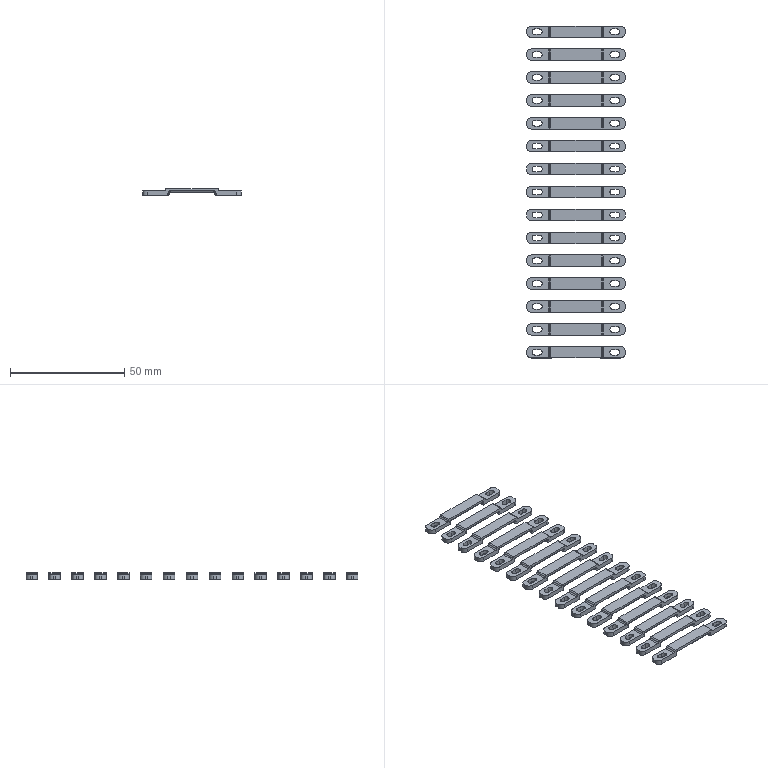NC program | NX | posted with a generic post | part box 43 x 145 x 3 mm
Whole program:
N10 G17 G21 G94 G90
(FLOOR_WALL_COPY , TOOL : D10JING)
N12 T15 M6
N14 G54
N16 G17 G0 G90 X29.5 Y0. S6500 M3
N18 G43 Z30. H15
N20 Z3.
N22 G94 G1 Z0. F1500.
N24 X26.5
N26 X-26.5
N28 X-29.5
N30 Z3.
N32 G0 Z30.
N34 M5
(FLOOR_WALL_1_COPY_1 , TOOL : D4)
N36 T11 M6
N38 G54
N40 G17 G0 G90 X-24.409 Y-1.452 S9500 M3
N42 G43 Z30. H11
N44 Z1.075
N46 G94 G1 Z0.075 F1000.
N48 X-23.643 Y-0.81
N50 G3 X-23.5 Y-0.503 R0.4
N52 G1 Y0.503 F2500.
N54 G2 X-21.075 Y4.177 R4.
N56 G1 Y-4.177
N58 G3 X-19.5 Y-4.5 R4.
N60 G1 X-18.65
N62 Y4.5
N64 X-16.225
N66 Y-4.5
N68 X-13.8
N70 Y4.5
N72 G3 X-13.943 Y4.806 R0.4
N74 G1 X-14.769 Y5.5
N76 Z1.075
N78 G0 X-24.409 Y-1.452 Z0.75
N80 G1 Z-0.25 F1000.
N82 X-23.643 Y-0.81
N84 G3 X-23.5 Y-0.503 R0.4
N86 G1 Y0.503 F2500.
N88 G2 X-21.075 Y4.177 R4.
N90 G1 Y-4.177
N92 G3 X-19.5 Y-4.5 R4.
N94 G1 X-18.65
N96 Y4.5
N98 X-16.225
N100 Y-4.5
N102 X-13.8
N104 Y4.5
N106 G3 X-13.943 Y4.806 R0.4
N108 G1 X-14.769 Y5.5
N110 Z0.75
N112 G0 X-24.409 Y-1.452 Z0.425
N114 G1 Z-0.575 F1000.
N116 X-23.643 Y-0.81
N118 G3 X-23.5 Y-0.503 R0.4
N120 G1 Y0.503 F2500.
N122 G2 X-21.075 Y4.177 R4.
N124 G1 Y-4.177
N126 G3 X-19.5 Y-4.5 R4.
N128 G1 X-18.65
N130 Y4.5
N132 X-16.225
N134 Y-4.5
N136 X-13.8
N138 Y4.5
N140 G3 X-13.943 Y4.806 R0.4
N142 G1 X-14.769 Y5.5
N144 Z0.425
N146 G0 Z30.
N148 X-24.402 Y-1.484
N150 Z0.1
N152 G1 Z-0.9 F1000.
N154 X-23.641 Y-0.836
N156 G3 X-23.5 Y-0.529 R0.4
N158 G1 Y-0.521 F2500.
N160 Y-0.5
N162 Y0.5
N164 G2 X-21.228 Y4.108 R4.
N166 G1 X-21.176 Y-4.132
N168 G3 X-19.5 Y-4.5 R4.
N170 G1 X-18.872
N172 X-18.929 Y4.5
N174 X-16.628
N176 X-16.571 Y-4.5
N178 X-14.269
N180 X-14.279 Y-2.97
N182 G3 X-14.424 Y-2.664 R0.4
N184 G1 X-14.8 Y-5.5
N186 Z0.1
N188 G0 Z30.
N190 X-14.322 Y-0.35
N192 Z0.425
N194 G1 X-14.3 Y2.922 Z-0.452 F1000.
N196 X-13.976 Y3.233 Z-0.572
N198 X-13.8 Y3.231 Z-0.619
N200 X-13.976 Y3.233 Z-0.666
N202 X-14.3 Y2.922 Z-0.787
N204 X-14.314 Y2.5 Z-0.9
N206 X-14.326 Y4.5 F2500.
N208 G3 X-14.471 Y4.806 R0.4
N210 G1 X-15.309 Y5.5
N212 Z0.1
N214 G0 Z30.
N216 X24.409 Y1.452
N218 Z1.075
N220 G1 Z0.075 F1000.
N222 X23.643 Y0.81
N224 G3 X23.5 Y0.503 R0.4
N226 G1 Y-0.503 F2500.
N228 G2 X21.075 Y-4.177 R4.
N230 G1 Y4.177
N232 G3 X19.5 Y4.5 R4.
N234 G1 X18.65
N236 Y-4.5
N238 X16.225
N240 Y4.5
N242 X13.8
N244 Y-4.5
N246 G3 X13.943 Y-4.806 R0.4
N248 G1 X14.769 Y-5.5
N250 Z1.075
N252 G0 X24.409 Y1.452 Z0.75
N254 G1 Z-0.25 F1000.
N256 X23.643 Y0.81
N258 G3 X23.5 Y0.503 R0.4
N260 G1 Y-0.503 F2500.
N262 G2 X21.075 Y-4.177 R4.
N264 G1 Y4.177
N266 G3 X19.5 Y4.5 R4.
N268 G1 X18.65
N270 Y-4.5
N272 X16.225
N274 Y4.5
N276 X13.8
N278 Y-4.5
N280 G3 X13.943 Y-4.806 R0.4
N282 G1 X14.769 Y-5.5
N284 Z0.75
N286 G0 X24.409 Y1.452 Z0.425
N288 G1 Z-0.575 F1000.
N290 X23.643 Y0.81
N292 G3 X23.5 Y0.503 R0.4
N294 G1 Y-0.503 F2500.
N296 G2 X21.075 Y-4.177 R4.
N298 G1 Y4.177
N300 G3 X19.5 Y4.5 R4.
N302 G1 X18.65
N304 Y-4.5
N306 X16.225
N308 Y4.5
N310 X13.8
N312 Y-4.5
N314 G3 X13.943 Y-4.806 R0.4
N316 G1 X14.769 Y-5.5
N318 Z0.425
N320 G0 Z30.
N322 X24.401 Y1.491
N324 Z0.1
N326 G1 Z-0.9 F1000.
N328 X23.64 Y0.843
N330 G3 X23.5 Y0.535 R0.4
N332 G1 Y0.528 F2500.
N334 Y0.5
N336 Y-0.5
N338 G2 X21.234 Y-4.104 R4.
N340 G1 X21.169 Y4.135
N342 G3 X19.5 Y4.5 R4.
N344 G1 X18.864
N346 X18.935 Y-4.5
N348 X16.633
N350 X16.562 Y4.5
N352 X14.26
N354 X14.272 Y2.958
N356 G3 X14.418 Y2.652 R0.4
N358 G1 X14.8 Y5.5
N360 Z0.1
N362 G0 Z30.
N364 X14.347 Y0.21
N366 Z0.425
N368 G1 X14.315 Y-2.5 Z-0.301 F1000.
N370 X14.287 Y-3.011 Z-0.438
N372 X13.976 Y-3.307 Z-0.554
N374 X13.8 Y-3.308 Z-0.601
N376 X13.976 Y-3.307 Z-0.648
N378 X14.287 Y-3.011 Z-0.763
N380 X14.315 Y-2.5 Z-0.9
N382 X14.331 Y-4.5 F2500.
N384 G3 X14.476 Y-4.805 R0.4
N386 G1 X15.318 Y-5.5
N388 Z0.1
N390 G0 Z30.
(FLOOR_WALL_1_COPY_COPY , TOOL : D4)
N392 X-24.409 Y-1.452
N394 Z0.
N396 G1 Z-1. F1000.
N398 X-23.643 Y-0.81
N400 G3 X-23.5 Y-0.503 R0.4
N402 G1 Y0.503 F1500.
N404 G2 X-21.6 Y3.904 R4.
N406 G1 Y-3.904
N408 G3 X-19.7 Y-4.495 R4.
N410 G1 Y4.495
N412 G2 X-19.5 Y4.5 R4.
N414 G1 X-17.8
N416 Y-4.5
N418 X-15.9
N420 Y4.5
N422 X-14.
N424 Y-4.5
N426 G2 X-14.143 Y-4.806 R0.4
N428 G1 X-14.969 Y-5.5
N430 Z0.
N432 G0 Z30.
N434 X24.409 Y1.452
N436 Z0.
N438 G1 Z-1. F1000.
N440 X23.643 Y0.81
N442 G3 X23.5 Y0.503 R0.4
N444 G1 Y-0.503 F1500.
N446 G2 X21.6 Y-3.904 R4.
N448 G1 Y3.904
N450 G3 X19.7 Y4.495 R4.
N452 G1 Y-4.495
N454 G2 X19.5 Y-4.5 R4.
N456 G1 X17.8
N458 Y4.5
N460 X15.9
N462 Y-4.5
N464 X14.
N466 Y4.5
N468 G2 X14.143 Y4.806 R0.4
N470 G1 X14.969 Y5.5
N472 Z0.
N474 G0 Z30.
N476 M5
(ZLEVEL_PROFILE_COPY_COPY_COPY_15 , TOOL : D2R0.5)
N478 T16 M6
N480 G54
N482 G17 G0 G90 X12.029 Y2.811 S9500 M3
N484 G43 Z30. H16
N486 Z0.982
N488 G94 G1 Z-0.018 F1000.
N490 X11.79 Y2.673
N492 G3 X11.69 Y2.5 R0.2
N494 G1 Y-2.5 F2500.
N496 X11.738 Z-0.031
N498 X11.794 Z-0.044
N500 Y2.5
N502 X11.847 Z-0.062
N504 X11.892 Z-0.08
N506 Y-2.5
N508 X11.936 Z-0.102
N510 X11.984 Z-0.125
N512 Y2.5
N514 X12.029 Z-0.152
N516 X12.07 Z-0.178
N518 Y-2.5
N520 X12.108 Z-0.209
N522 X12.15 Z-0.24
N524 Y2.5
N526 X12.188 Z-0.275
N528 X12.223 Z-0.309
N530 Y-2.5
N532 X12.254 Z-0.347
N534 X12.289 Z-0.385
N536 Y2.5
N538 X12.319 Z-0.426
N540 X12.346 Z-0.467
N542 Y-2.5
N544 X12.369 Z-0.511
N546 X12.395 Z-0.555
N548 Y2.5
N550 X12.417 Z-0.601
N552 X12.436 Z-0.647
N554 Y-2.5
N556 X12.446 Z-0.691
N558 X12.464 Z-0.735
N560 Y2.5
N562 X12.475 Z-0.779
N564 X12.484 Z-0.823
N566 Y-2.5
N568 X12.491 Z-0.868
N570 X12.496 Z-0.912
N572 Y2.5
N574 X12.5 Y2.474 Z-1.
N576 Y-2.473
N578 G3 X12.683 Y-2.553 R0.2
N580 G1 X12.912 Y-2.528
N582 Z0.
N584 G0 Z30.
N586 X-12.029 Y-2.811
N588 Z0.982
N590 G1 Z-0.018 F1000.
N592 X-11.79 Y-2.673
N594 G3 X-11.69 Y-2.5 R0.2
N596 G1 Y2.5 F2500.
N598 X-11.748 Z-0.031
N600 X-11.794 Z-0.044
N602 Y-2.5
N604 X-11.847 Z-0.062
N606 X-11.892 Z-0.08
N608 Y2.5
N610 X-11.941 Z-0.102
N612 X-11.984 Z-0.125
N614 Y-2.5
N616 X-12.029 Z-0.152
N618 X-12.07 Z-0.178
N620 Y2.5
N622 X-12.112 Z-0.209
N624 X-12.15 Z-0.24
N626 Y-2.5
N628 X-12.188 Z-0.275
N630 X-12.223 Z-0.309
N632 Y2.5
N634 X-12.258 Z-0.347
N636 X-12.289 Z-0.385
N638 Y-2.5
N640 X-12.319 Z-0.426
N642 X-12.346 Z-0.467
N644 Y2.5
N646 X-12.372 Z-0.511
N648 X-12.395 Z-0.555
N650 Y-2.5
N652 X-12.417 Z-0.601
N654 X-12.436 Z-0.647
N656 Y2.5
N658 X-12.451 Z-0.691
N660 X-12.464 Z-0.735
N662 Y-2.5
N664 X-12.475 Z-0.779
N666 X-12.484 Z-0.823
N668 Y2.5
N670 X-12.491 Z-0.868
N672 X-12.496 Z-0.912
N674 Y-2.5
N676 X-12.5 Y-2.475 Z-1.
N678 Y2.473
N680 G3 X-12.683 Y2.553 R0.2
N682 G1 X-12.913 Y2.528
N684 Z0.
N686 G0 Z30.
N688 M5
(PLANAR_MILL_COPY_COPY_COPY_COPY_COPY_COPY_1_COPY , TOOL : D6A45)
N690 T01 M6
N692 G54
N694 G17 G0 G90 X11.866 Y-3.9 S9500 M3
N696 G43 Z30. H1
N698 Z0.5
N700 G94 G1 Z-1. F1250.
N702 G3 X11. Y-3.4 R1.
N704 G1 X-11.
N706 G3 X-11.866 Y-3.9 R1.
N708 G1 Z0.5
N710 G0 Z30.
N712 Y3.9
N714 Z0.5
N716 G1 Z-1.
N718 G3 X-11. Y3.4 R1.
N720 G1 X11.
N722 G3 X11.866 Y3.9 R1.
N724 G1 Z0.5
N726 G0 Z30.
(PLANAR_MILL_COPY_COPY_COPY_COPY_COPY_COPY_1_COPY_COPY , TOOL : D6A45)
N728 X-18.02 Y-0.8
N730 Z0.
N732 G1 X-15.779 Z-0.601
N734 X-15.413 Y-0.587 Z-0.714
N736 X-15.2 Y-0.221 Z-0.827
N738 Y0.221 Z-0.946
N740 X-15.413 Y0.587 Z-1.059
N742 X-15.779 Y0.8 Z-1.173
N744 X-17. Z-1.5
N746 X-18.
N748 G3 X-18.8 Y0. R0.8
N750 X-18. Y-0.8 R0.8
N752 G1 X-16.
N754 G3 X-15.2 Y0. R0.8
N756 X-16. Y0.8 R0.8
N758 G1 X-17.
N760 G3 X-17.866 Y0.3 R1.
N762 G1 Z0.
N764 G0 Z30.
N766 X-14.697 Y-4.222
N768 Z0.
N770 G1 Z-1.5
N772 X-14.276 Y-3.849
N774 G3 X-13.96 Y-2.9 R1.
N776 G1 X-19.5
N778 G2 X-21.9 Y-0.5 R2.4
N780 G1 Y0.5
N782 G2 X-19.5 Y2.9 R2.4
N784 G1 X-13.96
N786 G3 X-14.276 Y3.849 R1.
N788 G1 X-14.697 Y4.222
N790 Z0.
N792 G0 Z30.
N794 X14.697
N796 Z0.
N798 G1 Z-1.5
N800 X14.276 Y3.849
N802 G3 X13.96 Y2.9 R1.
N804 G1 X19.5
N806 G2 X21.9 Y0.5 R2.4
N808 G1 Y-0.5
N810 G2 X19.5 Y-2.9 R2.4
N812 G1 X13.96
N814 G3 X14.276 Y-3.849 R1.
N816 G1 X14.697 Y-4.222
N818 Z0.
N820 G0 Z30.
N822 X15.98 Y-0.8
N824 Z0.
N826 G1 X18.221 Z-0.601
N828 X18.587 Y-0.587 Z-0.714
N830 X18.8 Y-0.221 Z-0.827
N832 Y0.221 Z-0.946
N834 X18.587 Y0.587 Z-1.059
N836 X18.221 Y0.8 Z-1.173
N838 X17. Z-1.5
N840 X16.
N842 G3 X15.2 Y0. R0.8
N844 X16. Y-0.8 R0.8
N846 G1 X18.
N848 G3 X18.8 Y0. R0.8
N850 X18. Y0.8 R0.8
N852 G1 X17.
N854 G3 X16.134 Y0.3 R1.
N856 G1 Z0.
N858 G0 Z30.
N860 M5
N862 M2